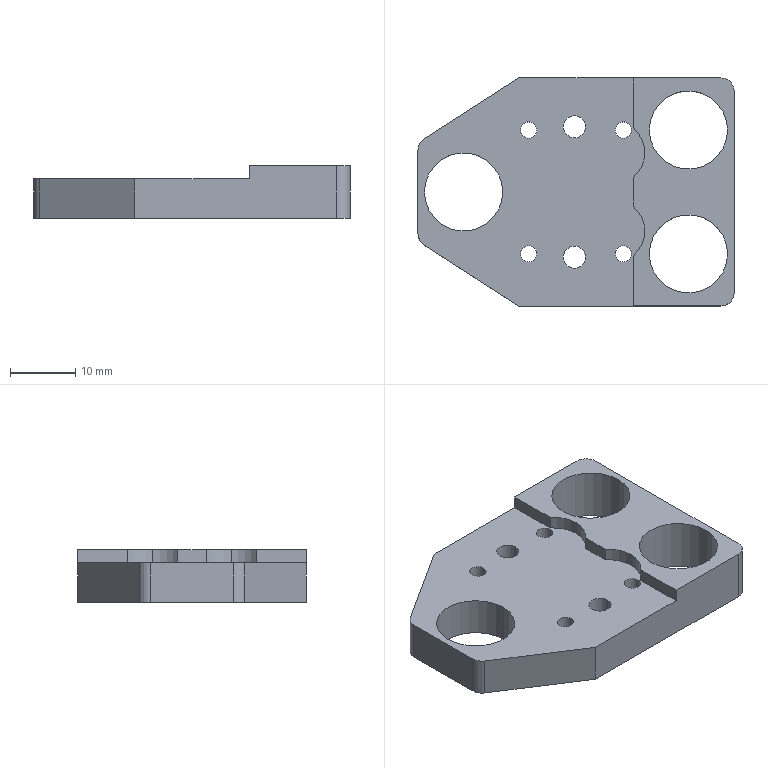Part | STEP file | 11-FG-SB00411 | 1 solid | 44 faces | box 48.5 x 35 x 8 mm | volume 7407 mm3 | cylinder 30 | plane 14 | commonest cylinder face diameters 2.5 x8 12 x6 3.4 x4 4 x4 6.5 x4 10 x4
STEP:
#1=CARTESIAN_POINT('',(-13.75,-9.5,6.));
#2=VERTEX_POINT('',#1);
#3=CARTESIAN_POINT('',(-16.25,-9.5,6.));
#4=VERTEX_POINT('',#3);
#5=CARTESIAN_POINT('',(-15.,-9.5,6.));
#6=DIRECTION('',(0.,0.,-1.));
#7=DIRECTION('',(-1.,0.,0.));
#8=AXIS2_PLACEMENT_3D('',#5,#6,#7);
#9=CIRCLE('',#8,1.25);
#10=EDGE_CURVE('',#2,#4,#9,.T.);
#11=ORIENTED_EDGE('',*,*,#10,.F.);
#12=CARTESIAN_POINT('',(-13.75,-9.5,0.));
#13=VERTEX_POINT('',#12);
#14=CARTESIAN_POINT('',(-13.75,-9.5,0.));
#15=DIRECTION('',(0.,0.,-1.));
#16=VECTOR('',#15,1000.);
#17=LINE('',#14,#16);
#18=EDGE_CURVE('',#2,#13,#17,.T.);
#19=ORIENTED_EDGE('',*,*,#18,.T.);
#20=CARTESIAN_POINT('',(-16.25,-9.5,0.));
#21=VERTEX_POINT('',#20);
#22=CARTESIAN_POINT('',(-15.,-9.5,0.));
#23=DIRECTION('',(0.,0.,-1.));
#24=DIRECTION('',(-1.,0.,0.));
#25=AXIS2_PLACEMENT_3D('',#22,#23,#24);
#26=CIRCLE('',#25,1.25);
#27=EDGE_CURVE('',#13,#21,#26,.T.);
#28=ORIENTED_EDGE('',*,*,#27,.T.);
#29=CARTESIAN_POINT('',(-16.25,-9.5,0.));
#30=DIRECTION('',(0.,0.,-1.));
#31=VECTOR('',#30,1000.);
#32=LINE('',#29,#31);
#33=EDGE_CURVE('',#4,#21,#32,.T.);
#34=ORIENTED_EDGE('',*,*,#33,.F.);
#35=EDGE_LOOP('',(#11,#19,#28,#34));
#36=FACE_OUTER_BOUND('',#35,.T.);
#37=CARTESIAN_POINT('',(-15.,-9.5,0.));
#38=DIRECTION('',(0.,0.,-1.));
#39=DIRECTION('',(-1.,0.,0.));
#40=AXIS2_PLACEMENT_3D('',#37,#38,#39);
#41=CYLINDRICAL_SURFACE('',#40,1.25);
#42=ADVANCED_FACE('',(#36),#41,.F.);
#43=CARTESIAN_POINT('',(-13.75,9.5,6.));
#44=VERTEX_POINT('',#43);
#45=CARTESIAN_POINT('',(-16.25,9.5,6.));
#46=VERTEX_POINT('',#45);
#47=CARTESIAN_POINT('',(-15.,9.5,6.));
#48=DIRECTION('',(0.,0.,-1.));
#49=DIRECTION('',(-1.,0.,0.));
#50=AXIS2_PLACEMENT_3D('',#47,#48,#49);
#51=CIRCLE('',#50,1.25);
#52=EDGE_CURVE('',#44,#46,#51,.T.);
#53=ORIENTED_EDGE('',*,*,#52,.F.);
#54=CARTESIAN_POINT('',(-13.75,9.5,0.));
#55=VERTEX_POINT('',#54);
#56=CARTESIAN_POINT('',(-13.75,9.5,0.));
#57=DIRECTION('',(0.,0.,-1.));
#58=VECTOR('',#57,1000.);
#59=LINE('',#56,#58);
#60=EDGE_CURVE('',#44,#55,#59,.T.);
#61=ORIENTED_EDGE('',*,*,#60,.T.);
#62=CARTESIAN_POINT('',(-16.25,9.5,0.));
#63=VERTEX_POINT('',#62);
#64=CARTESIAN_POINT('',(-15.,9.5,0.));
#65=DIRECTION('',(0.,0.,-1.));
#66=DIRECTION('',(-1.,0.,0.));
#67=AXIS2_PLACEMENT_3D('',#64,#65,#66);
#68=CIRCLE('',#67,1.25);
#69=EDGE_CURVE('',#55,#63,#68,.T.);
#70=ORIENTED_EDGE('',*,*,#69,.T.);
#71=CARTESIAN_POINT('',(-16.25,9.5,0.));
#72=DIRECTION('',(0.,0.,-1.));
#73=VECTOR('',#72,1000.);
#74=LINE('',#71,#73);
#75=EDGE_CURVE('',#46,#63,#74,.T.);
#76=ORIENTED_EDGE('',*,*,#75,.F.);
#77=EDGE_LOOP('',(#53,#61,#70,#76));
#78=FACE_OUTER_BOUND('',#77,.T.);
#79=CARTESIAN_POINT('',(-15.,9.5,0.));
#80=DIRECTION('',(0.,0.,-1.));
#81=DIRECTION('',(-1.,0.,0.));
#82=AXIS2_PLACEMENT_3D('',#79,#80,#81);
#83=CYLINDRICAL_SURFACE('',#82,1.25);
#84=ADVANCED_FACE('',(#78),#83,.F.);
#85=CARTESIAN_POINT('',(-31.,0.,0.));
#86=VERTEX_POINT('',#85);
#87=CARTESIAN_POINT('',(-19.,0.,0.));
#88=VERTEX_POINT('',#87);
#89=CARTESIAN_POINT('',(-25.,0.,0.));
#90=DIRECTION('',(0.,0.,1.));
#91=DIRECTION('',(1.,0.,0.));
#92=AXIS2_PLACEMENT_3D('',#89,#90,#91);
#93=CIRCLE('',#92,6.);
#94=EDGE_CURVE('',#86,#88,#93,.T.);
#95=ORIENTED_EDGE('',*,*,#94,.F.);
#96=CARTESIAN_POINT('',(-31.,0.,6.));
#97=VERTEX_POINT('',#96);
#98=CARTESIAN_POINT('',(-31.,0.,0.));
#99=DIRECTION('',(0.,0.,1.));
#100=VECTOR('',#99,1000.);
#101=LINE('',#98,#100);
#102=EDGE_CURVE('',#86,#97,#101,.T.);
#103=ORIENTED_EDGE('',*,*,#102,.T.);
#104=CARTESIAN_POINT('',(-19.,0.,6.));
#105=VERTEX_POINT('',#104);
#106=CARTESIAN_POINT('',(-25.,0.,6.));
#107=DIRECTION('',(0.,0.,1.));
#108=DIRECTION('',(1.,0.,0.));
#109=AXIS2_PLACEMENT_3D('',#106,#107,#108);
#110=CIRCLE('',#109,6.);
#111=EDGE_CURVE('',#97,#105,#110,.T.);
#112=ORIENTED_EDGE('',*,*,#111,.T.);
#113=CARTESIAN_POINT('',(-19.,0.,0.));
#114=DIRECTION('',(0.,0.,1.));
#115=VECTOR('',#114,1000.);
#116=LINE('',#113,#115);
#117=EDGE_CURVE('',#88,#105,#116,.T.);
#118=ORIENTED_EDGE('',*,*,#117,.F.);
#119=EDGE_LOOP('',(#95,#103,#112,#118));
#120=FACE_OUTER_BOUND('',#119,.T.);
#121=CARTESIAN_POINT('',(-25.,0.,0.));
#122=DIRECTION('',(0.,0.,1.));
#123=DIRECTION('',(1.,0.,0.));
#124=AXIS2_PLACEMENT_3D('',#121,#122,#123);
#125=CYLINDRICAL_SURFACE('',#124,6.);
#126=ADVANCED_FACE('',(#120),#125,.F.);
#127=CARTESIAN_POINT('',(0.75,-9.5,6.));
#128=VERTEX_POINT('',#127);
#129=CARTESIAN_POINT('',(-1.75,-9.5,6.));
#130=VERTEX_POINT('',#129);
#131=CARTESIAN_POINT('',(-0.5,-9.5,6.));
#132=DIRECTION('',(0.,0.,-1.));
#133=DIRECTION('',(-1.,0.,0.));
#134=AXIS2_PLACEMENT_3D('',#131,#132,#133);
#135=CIRCLE('',#134,1.25);
#136=EDGE_CURVE('',#128,#130,#135,.T.);
#137=ORIENTED_EDGE('',*,*,#136,.F.);
#138=CARTESIAN_POINT('',(0.75,-9.5,0.));
#139=VERTEX_POINT('',#138);
#140=CARTESIAN_POINT('',(0.75,-9.5,0.));
#141=DIRECTION('',(0.,0.,-1.));
#142=VECTOR('',#141,1000.);
#143=LINE('',#140,#142);
#144=EDGE_CURVE('',#128,#139,#143,.T.);
#145=ORIENTED_EDGE('',*,*,#144,.T.);
#146=CARTESIAN_POINT('',(-1.75,-9.5,0.));
#147=VERTEX_POINT('',#146);
#148=CARTESIAN_POINT('',(-0.5,-9.5,0.));
#149=DIRECTION('',(0.,0.,-1.));
#150=DIRECTION('',(-1.,0.,0.));
#151=AXIS2_PLACEMENT_3D('',#148,#149,#150);
#152=CIRCLE('',#151,1.25);
#153=EDGE_CURVE('',#139,#147,#152,.T.);
#154=ORIENTED_EDGE('',*,*,#153,.T.);
#155=CARTESIAN_POINT('',(-1.75,-9.5,0.));
#156=DIRECTION('',(0.,0.,-1.));
#157=VECTOR('',#156,1000.);
#158=LINE('',#155,#157);
#159=EDGE_CURVE('',#130,#147,#158,.T.);
#160=ORIENTED_EDGE('',*,*,#159,.F.);
#161=EDGE_LOOP('',(#137,#145,#154,#160));
#162=FACE_OUTER_BOUND('',#161,.T.);
#163=CARTESIAN_POINT('',(-0.5,-9.5,0.));
#164=DIRECTION('',(0.,0.,-1.));
#165=DIRECTION('',(-1.,0.,0.));
#166=AXIS2_PLACEMENT_3D('',#163,#164,#165);
#167=CYLINDRICAL_SURFACE('',#166,1.25);
#168=ADVANCED_FACE('',(#162),#167,.F.);
#169=CARTESIAN_POINT('',(0.75,9.5,6.));
#170=VERTEX_POINT('',#169);
#171=CARTESIAN_POINT('',(-1.75,9.5,6.));
#172=VERTEX_POINT('',#171);
#173=CARTESIAN_POINT('',(-0.5,9.5,6.));
#174=DIRECTION('',(0.,0.,-1.));
#175=DIRECTION('',(-1.,0.,0.));
#176=AXIS2_PLACEMENT_3D('',#173,#174,#175);
#177=CIRCLE('',#176,1.25);
#178=EDGE_CURVE('',#170,#172,#177,.T.);
#179=ORIENTED_EDGE('',*,*,#178,.F.);
#180=CARTESIAN_POINT('',(0.75,9.5,0.));
#181=VERTEX_POINT('',#180);
#182=CARTESIAN_POINT('',(0.75,9.5,0.));
#183=DIRECTION('',(0.,0.,-1.));
#184=VECTOR('',#183,1000.);
#185=LINE('',#182,#184);
#186=EDGE_CURVE('',#170,#181,#185,.T.);
#187=ORIENTED_EDGE('',*,*,#186,.T.);
#188=CARTESIAN_POINT('',(-1.75,9.5,0.));
#189=VERTEX_POINT('',#188);
#190=CARTESIAN_POINT('',(-0.5,9.5,0.));
#191=DIRECTION('',(0.,0.,-1.));
#192=DIRECTION('',(-1.,0.,0.));
#193=AXIS2_PLACEMENT_3D('',#190,#191,#192);
#194=CIRCLE('',#193,1.25);
#195=EDGE_CURVE('',#181,#189,#194,.T.);
#196=ORIENTED_EDGE('',*,*,#195,.T.);
#197=CARTESIAN_POINT('',(-1.75,9.5,0.));
#198=DIRECTION('',(0.,0.,-1.));
#199=VECTOR('',#198,1000.);
#200=LINE('',#197,#199);
#201=EDGE_CURVE('',#172,#189,#200,.T.);
#202=ORIENTED_EDGE('',*,*,#201,.F.);
#203=EDGE_LOOP('',(#179,#187,#196,#202));
#204=FACE_OUTER_BOUND('',#203,.T.);
#205=CARTESIAN_POINT('',(-0.5,9.5,0.));
#206=DIRECTION('',(0.,0.,-1.));
#207=DIRECTION('',(-1.,0.,0.));
#208=AXIS2_PLACEMENT_3D('',#205,#206,#207);
#209=CYLINDRICAL_SURFACE('',#208,1.25);
#210=ADVANCED_FACE('',(#204),#209,.F.);
#211=CARTESIAN_POINT('',(3.5,9.5,0.));
#212=VERTEX_POINT('',#211);
#213=CARTESIAN_POINT('',(15.5,9.5,0.));
#214=VERTEX_POINT('',#213);
#215=CARTESIAN_POINT('',(9.5,9.5,0.));
#216=DIRECTION('',(0.,0.,1.));
#217=DIRECTION('',(-1.,0.,0.));
#218=AXIS2_PLACEMENT_3D('',#215,#216,#217);
#219=CIRCLE('',#218,6.);
#220=EDGE_CURVE('',#212,#214,#219,.T.);
#221=ORIENTED_EDGE('',*,*,#220,.F.);
#222=CARTESIAN_POINT('',(3.5,9.5,8.));
#223=VERTEX_POINT('',#222);
#224=CARTESIAN_POINT('',(3.5,9.5,0.));
#225=DIRECTION('',(0.,0.,1.));
#226=VECTOR('',#225,1000.);
#227=LINE('',#224,#226);
#228=EDGE_CURVE('',#212,#223,#227,.T.);
#229=ORIENTED_EDGE('',*,*,#228,.T.);
#230=CARTESIAN_POINT('',(15.5,9.5,8.));
#231=VERTEX_POINT('',#230);
#232=CARTESIAN_POINT('',(9.5,9.5,8.));
#233=DIRECTION('',(0.,0.,1.));
#234=DIRECTION('',(-1.,0.,0.));
#235=AXIS2_PLACEMENT_3D('',#232,#233,#234);
#236=CIRCLE('',#235,6.);
#237=EDGE_CURVE('',#223,#231,#236,.T.);
#238=ORIENTED_EDGE('',*,*,#237,.T.);
#239=CARTESIAN_POINT('',(15.5,9.5,0.));
#240=DIRECTION('',(0.,0.,1.));
#241=VECTOR('',#240,1000.);
#242=LINE('',#239,#241);
#243=EDGE_CURVE('',#214,#231,#242,.T.);
#244=ORIENTED_EDGE('',*,*,#243,.F.);
#245=EDGE_LOOP('',(#221,#229,#238,#244));
#246=FACE_OUTER_BOUND('',#245,.T.);
#247=CARTESIAN_POINT('',(9.5,9.5,0.));
#248=DIRECTION('',(0.,0.,1.));
#249=DIRECTION('',(1.,0.,0.));
#250=AXIS2_PLACEMENT_3D('',#247,#248,#249);
#251=CYLINDRICAL_SURFACE('',#250,6.);
#252=ADVANCED_FACE('',(#246),#251,.F.);
#253=CARTESIAN_POINT('',(3.5,-9.5,0.));
#254=VERTEX_POINT('',#253);
#255=CARTESIAN_POINT('',(15.5,-9.5,0.));
#256=VERTEX_POINT('',#255);
#257=CARTESIAN_POINT('',(9.5,-9.5,0.));
#258=DIRECTION('',(0.,0.,1.));
#259=DIRECTION('',(1.,0.,0.));
#260=AXIS2_PLACEMENT_3D('',#257,#258,#259);
#261=CIRCLE('',#260,6.);
#262=EDGE_CURVE('',#254,#256,#261,.T.);
#263=ORIENTED_EDGE('',*,*,#262,.F.);
#264=CARTESIAN_POINT('',(3.5,-9.5,8.));
#265=VERTEX_POINT('',#264);
#266=CARTESIAN_POINT('',(3.5,-9.5,0.));
#267=DIRECTION('',(0.,0.,1.));
#268=VECTOR('',#267,1000.);
#269=LINE('',#266,#268);
#270=EDGE_CURVE('',#254,#265,#269,.T.);
#271=ORIENTED_EDGE('',*,*,#270,.T.);
#272=CARTESIAN_POINT('',(15.5,-9.5,8.));
#273=VERTEX_POINT('',#272);
#274=CARTESIAN_POINT('',(9.5,-9.5,8.));
#275=DIRECTION('',(0.,0.,1.));
#276=DIRECTION('',(1.,0.,0.));
#277=AXIS2_PLACEMENT_3D('',#274,#275,#276);
#278=CIRCLE('',#277,6.);
#279=EDGE_CURVE('',#265,#273,#278,.T.);
#280=ORIENTED_EDGE('',*,*,#279,.T.);
#281=CARTESIAN_POINT('',(15.5,-9.5,0.));
#282=DIRECTION('',(0.,0.,1.));
#283=VECTOR('',#282,1000.);
#284=LINE('',#281,#283);
#285=EDGE_CURVE('',#256,#273,#284,.T.);
#286=ORIENTED_EDGE('',*,*,#285,.F.);
#287=EDGE_LOOP('',(#263,#271,#280,#286));
#288=FACE_OUTER_BOUND('',#287,.T.);
#289=CARTESIAN_POINT('',(9.5,-9.5,0.));
#290=DIRECTION('',(0.,0.,1.));
#291=DIRECTION('',(1.,0.,0.));
#292=AXIS2_PLACEMENT_3D('',#289,#290,#291);
#293=CYLINDRICAL_SURFACE('',#292,6.);
#294=ADVANCED_FACE('',(#288),#293,.F.);
#295=CARTESIAN_POINT('',(-4.75,-10.,3.4));
#296=VERTEX_POINT('',#295);
#297=CARTESIAN_POINT('',(-11.25,-10.,3.4));
#298=VERTEX_POINT('',#297);
#299=CARTESIAN_POINT('',(-8.,-10.,3.4));
#300=DIRECTION('',(0.,0.,-1.));
#301=DIRECTION('',(-1.,0.,0.));
#302=AXIS2_PLACEMENT_3D('',#299,#300,#301);
#303=CIRCLE('',#302,3.25);
#304=EDGE_CURVE('',#296,#298,#303,.T.);
#305=ORIENTED_EDGE('',*,*,#304,.F.);
#306=CARTESIAN_POINT('',(-4.75,-10.,0.));
#307=VERTEX_POINT('',#306);
#308=CARTESIAN_POINT('',(-4.75,-10.,0.));
#309=DIRECTION('',(0.,0.,-1.));
#310=VECTOR('',#309,1000.);
#311=LINE('',#308,#310);
#312=EDGE_CURVE('',#296,#307,#311,.T.);
#313=ORIENTED_EDGE('',*,*,#312,.T.);
#314=CARTESIAN_POINT('',(-11.25,-10.,0.));
#315=VERTEX_POINT('',#314);
#316=CARTESIAN_POINT('',(-8.,-10.,0.));
#317=DIRECTION('',(0.,0.,-1.));
#318=DIRECTION('',(-1.,0.,0.));
#319=AXIS2_PLACEMENT_3D('',#316,#317,#318);
#320=CIRCLE('',#319,3.25);
#321=EDGE_CURVE('',#307,#315,#320,.T.);
#322=ORIENTED_EDGE('',*,*,#321,.T.);
#323=CARTESIAN_POINT('',(-11.25,-10.,0.));
#324=DIRECTION('',(0.,0.,-1.));
#325=VECTOR('',#324,1000.);
#326=LINE('',#323,#325);
#327=EDGE_CURVE('',#298,#315,#326,.T.);
#328=ORIENTED_EDGE('',*,*,#327,.F.);
#329=EDGE_LOOP('',(#305,#313,#322,#328));
#330=FACE_OUTER_BOUND('',#329,.T.);
#331=CARTESIAN_POINT('',(-8.,-10.,0.));
#332=DIRECTION('',(0.,0.,-1.));
#333=DIRECTION('',(-1.,0.,0.));
#334=AXIS2_PLACEMENT_3D('',#331,#332,#333);
#335=CYLINDRICAL_SURFACE('',#334,3.25);
#336=ADVANCED_FACE('',(#330),#335,.F.);
#337=CARTESIAN_POINT('',(-6.3,-10.,6.));
#338=VERTEX_POINT('',#337);
#339=CARTESIAN_POINT('',(-9.7,-10.,6.));
#340=VERTEX_POINT('',#339);
#341=CARTESIAN_POINT('',(-8.,-10.,6.));
#342=DIRECTION('',(0.,0.,-1.));
#343=DIRECTION('',(-1.,0.,0.));
#344=AXIS2_PLACEMENT_3D('',#341,#342,#343);
#345=CIRCLE('',#344,1.7);
#346=EDGE_CURVE('',#338,#340,#345,.T.);
#347=ORIENTED_EDGE('',*,*,#346,.F.);
#348=CARTESIAN_POINT('',(-6.3,-10.,3.4));
#349=VERTEX_POINT('',#348);
#350=CARTESIAN_POINT('',(-6.3,-10.,0.));
#351=DIRECTION('',(0.,0.,-1.));
#352=VECTOR('',#351,1000.);
#353=LINE('',#350,#352);
#354=EDGE_CURVE('',#338,#349,#353,.T.);
#355=ORIENTED_EDGE('',*,*,#354,.T.);
#356=CARTESIAN_POINT('',(-9.7,-10.,3.4));
#357=VERTEX_POINT('',#356);
#358=CARTESIAN_POINT('',(-8.,-10.,3.4));
#359=DIRECTION('',(0.,0.,-1.));
#360=DIRECTION('',(-1.,0.,0.));
#361=AXIS2_PLACEMENT_3D('',#358,#359,#360);
#362=CIRCLE('',#361,1.7);
#363=EDGE_CURVE('',#349,#357,#362,.T.);
#364=ORIENTED_EDGE('',*,*,#363,.T.);
#365=CARTESIAN_POINT('',(-9.7,-10.,0.));
#366=DIRECTION('',(0.,0.,-1.));
#367=VECTOR('',#366,1000.);
#368=LINE('',#365,#367);
#369=EDGE_CURVE('',#340,#357,#368,.T.);
#370=ORIENTED_EDGE('',*,*,#369,.F.);
#371=EDGE_LOOP('',(#347,#355,#364,#370));
#372=FACE_OUTER_BOUND('',#371,.T.);
#373=CARTESIAN_POINT('',(-8.,-10.,0.));
#374=DIRECTION('',(0.,0.,-1.));
#375=DIRECTION('',(-1.,0.,0.));
#376=AXIS2_PLACEMENT_3D('',#373,#374,#375);
#377=CYLINDRICAL_SURFACE('',#376,1.7);
#378=ADVANCED_FACE('',(#372),#377,.F.);
#379=CARTESIAN_POINT('',(-4.75,10.,3.4));
#380=VERTEX_POINT('',#379);
#381=CARTESIAN_POINT('',(-11.25,10.,3.4));
#382=VERTEX_POINT('',#381);
#383=CARTESIAN_POINT('',(-8.,10.,3.4));
#384=DIRECTION('',(0.,0.,-1.));
#385=DIRECTION('',(-1.,0.,0.));
#386=AXIS2_PLACEMENT_3D('',#383,#384,#385);
#387=CIRCLE('',#386,3.25);
#388=EDGE_CURVE('',#380,#382,#387,.T.);
#389=ORIENTED_EDGE('',*,*,#388,.F.);
#390=CARTESIAN_POINT('',(-4.75,10.,0.));
#391=VERTEX_POINT('',#390);
#392=CARTESIAN_POINT('',(-4.75,10.,0.));
#393=DIRECTION('',(0.,0.,-1.));
#394=VECTOR('',#393,1000.);
#395=LINE('',#392,#394);
#396=EDGE_CURVE('',#380,#391,#395,.T.);
#397=ORIENTED_EDGE('',*,*,#396,.T.);
#398=CARTESIAN_POINT('',(-11.25,10.,0.));
#399=VERTEX_POINT('',#398);
#400=CARTESIAN_POINT('',(-8.,10.,0.));
#401=DIRECTION('',(0.,0.,-1.));
#402=DIRECTION('',(-1.,0.,0.));
#403=AXIS2_PLACEMENT_3D('',#400,#401,#402);
#404=CIRCLE('',#403,3.25);
#405=EDGE_CURVE('',#391,#399,#404,.T.);
#406=ORIENTED_EDGE('',*,*,#405,.T.);
#407=CARTESIAN_POINT('',(-11.25,10.,0.));
#408=DIRECTION('',(0.,0.,-1.));
#409=VECTOR('',#408,1000.);
#410=LINE('',#407,#409);
#411=EDGE_CURVE('',#382,#399,#410,.T.);
#412=ORIENTED_EDGE('',*,*,#411,.F.);
#413=EDGE_LOOP('',(#389,#397,#406,#412));
#414=FACE_OUTER_BOUND('',#413,.T.);
#415=CARTESIAN_POINT('',(-8.,10.,0.));
#416=DIRECTION('',(0.,0.,-1.));
#417=DIRECTION('',(-1.,0.,0.));
#418=AXIS2_PLACEMENT_3D('',#415,#416,#417);
#419=CYLINDRICAL_SURFACE('',#418,3.25);
#420=ADVANCED_FACE('',(#414),#419,.F.);
#421=CARTESIAN_POINT('',(-6.3,10.,6.));
#422=VERTEX_POINT('',#421);
#423=CARTESIAN_POINT('',(-9.7,10.,6.));
#424=VERTEX_POINT('',#423);
#425=CARTESIAN_POINT('',(-8.,10.,6.));
#426=DIRECTION('',(0.,0.,-1.));
#427=DIRECTION('',(-1.,0.,0.));
#428=AXIS2_PLACEMENT_3D('',#425,#426,#427);
#429=CIRCLE('',#428,1.7);
#430=EDGE_CURVE('',#422,#424,#429,.T.);
#431=ORIENTED_EDGE('',*,*,#430,.F.);
#432=CARTESIAN_POINT('',(-6.3,10.,3.4));
#433=VERTEX_POINT('',#432);
#434=CARTESIAN_POINT('',(-6.3,10.,0.));
#435=DIRECTION('',(0.,0.,-1.));
#436=VECTOR('',#435,1000.);
#437=LINE('',#434,#436);
#438=EDGE_CURVE('',#422,#433,#437,.T.);
#439=ORIENTED_EDGE('',*,*,#438,.T.);
#440=CARTESIAN_POINT('',(-9.7,10.,3.4));
#441=VERTEX_POINT('',#440);
#442=CARTESIAN_POINT('',(-8.,10.,3.4));
#443=DIRECTION('',(0.,0.,-1.));
#444=DIRECTION('',(-1.,0.,0.));
#445=AXIS2_PLACEMENT_3D('',#442,#443,#444);
#446=CIRCLE('',#445,1.7);
#447=EDGE_CURVE('',#433,#441,#446,.T.);
#448=ORIENTED_EDGE('',*,*,#447,.T.);
#449=CARTESIAN_POINT('',(-9.7,10.,0.));
#450=DIRECTION('',(0.,0.,-1.));
#451=VECTOR('',#450,1000.);
#452=LINE('',#449,#451);
#453=EDGE_CURVE('',#424,#441,#452,.T.);
#454=ORIENTED_EDGE('',*,*,#453,.F.);
#455=EDGE_LOOP('',(#431,#439,#448,#454));
#456=FACE_OUTER_BOUND('',#455,.T.);
#457=CARTESIAN_POINT('',(-8.,10.,0.));
#458=DIRECTION('',(0.,0.,-1.));
#459=DIRECTION('',(-1.,0.,0.));
#460=AXIS2_PLACEMENT_3D('',#457,#458,#459);
#461=CYLINDRICAL_SURFACE('',#460,1.7);
#462=ADVANCED_FACE('',(#456),#461,.F.);
#463=CARTESIAN_POINT('',(2.8,-6.,6.));
#464=VERTEX_POINT('',#463);
#465=CARTESIAN_POINT('',(1.,-2.158,6.));
#466=VERTEX_POINT('',#465);
#467=CARTESIAN_POINT('',(-2.2,-6.,6.));
#468=DIRECTION('',(0.,0.,1.));
#469=DIRECTION('',(-1.,0.,0.));
#470=AXIS2_PLACEMENT_3D('',#467,#468,#469);
#471=CIRCLE('',#470,5.);
#472=EDGE_CURVE('',#464,#466,#471,.T.);
#473=ORIENTED_EDGE('',*,*,#472,.F.);
#474=CARTESIAN_POINT('',(2.8,-6.,8.));
#475=VERTEX_POINT('',#474);
#476=CARTESIAN_POINT('',(2.8,-6.,6.));
#477=DIRECTION('',(0.,0.,1.));
#478=VECTOR('',#477,1000.);
#479=LINE('',#476,#478);
#480=EDGE_CURVE('',#464,#475,#479,.T.);
#481=ORIENTED_EDGE('',*,*,#480,.T.);
#482=CARTESIAN_POINT('',(1.,-2.158,8.));
#483=VERTEX_POINT('',#482);
#484=CARTESIAN_POINT('',(-2.2,-6.,8.));
#485=DIRECTION('',(0.,0.,1.));
#486=DIRECTION('',(-1.,0.,0.));
#487=AXIS2_PLACEMENT_3D('',#484,#485,#486);
#488=CIRCLE('',#487,5.);
#489=EDGE_CURVE('',#475,#483,#488,.T.);
#490=ORIENTED_EDGE('',*,*,#489,.T.);
#491=CARTESIAN_POINT('',(1.,-2.158,6.));
#492=DIRECTION('',(0.,0.,1.));
#493=VECTOR('',#492,1000.);
#494=LINE('',#491,#493);
#495=EDGE_CURVE('',#466,#483,#494,.T.);
#496=ORIENTED_EDGE('',*,*,#495,.F.);
#497=EDGE_LOOP('',(#473,#481,#490,#496));
#498=FACE_OUTER_BOUND('',#497,.T.);
#499=CARTESIAN_POINT('',(-2.2,-6.,6.));
#500=DIRECTION('',(0.,0.,1.));
#501=DIRECTION('',(1.,0.,0.));
#502=AXIS2_PLACEMENT_3D('',#499,#500,#501);
#503=CYLINDRICAL_SURFACE('',#502,5.);
#504=ADVANCED_FACE('',(#498),#503,.F.);
#505=CARTESIAN_POINT('',(2.8,6.,6.));
#506=VERTEX_POINT('',#505);
#507=CARTESIAN_POINT('',(1.,9.842,6.));
#508=VERTEX_POINT('',#507);
#509=CARTESIAN_POINT('',(-2.2,6.,6.));
#510=DIRECTION('',(0.,0.,1.));
#511=DIRECTION('',(1.,0.,0.));
#512=AXIS2_PLACEMENT_3D('',#509,#510,#511);
#513=CIRCLE('',#512,5.);
#514=EDGE_CURVE('',#506,#508,#513,.T.);
#515=ORIENTED_EDGE('',*,*,#514,.F.);
#516=CARTESIAN_POINT('',(2.8,6.,8.));
#517=VERTEX_POINT('',#516);
#518=CARTESIAN_POINT('',(2.8,6.,6.));
#519=DIRECTION('',(0.,0.,1.));
#520=VECTOR('',#519,1000.);
#521=LINE('',#518,#520);
#522=EDGE_CURVE('',#506,#517,#521,.T.);
#523=ORIENTED_EDGE('',*,*,#522,.T.);
#524=CARTESIAN_POINT('',(1.,9.842,8.));
#525=VERTEX_POINT('',#524);
#526=CARTESIAN_POINT('',(-2.2,6.,8.));
#527=DIRECTION('',(0.,0.,1.));
#528=DIRECTION('',(1.,0.,0.));
#529=AXIS2_PLACEMENT_3D('',#526,#527,#528);
#530=CIRCLE('',#529,5.);
#531=EDGE_CURVE('',#517,#525,#530,.T.);
#532=ORIENTED_EDGE('',*,*,#531,.T.);
#533=CARTESIAN_POINT('',(1.,9.842,6.));
#534=DIRECTION('',(0.,0.,1.));
#535=VECTOR('',#534,1000.);
#536=LINE('',#533,#535);
#537=EDGE_CURVE('',#508,#525,#536,.T.);
#538=ORIENTED_EDGE('',*,*,#537,.F.);
#539=EDGE_LOOP('',(#515,#523,#532,#538));
#540=FACE_OUTER_BOUND('',#539,.T.);
#541=CARTESIAN_POINT('',(-2.2,6.,6.));
#542=DIRECTION('',(0.,0.,1.));
#543=DIRECTION('',(1.,0.,0.));
#544=AXIS2_PLACEMENT_3D('',#541,#542,#543);
#545=CYLINDRICAL_SURFACE('',#544,5.);
#546=ADVANCED_FACE('',(#540),#545,.F.);
#547=CARTESIAN_POINT('',(1.,2.158,6.));
#548=VERTEX_POINT('',#547);
#549=CARTESIAN_POINT('',(1.,17.5,6.));
#550=DIRECTION('',(0.,-1.,0.));
#551=VECTOR('',#550,1000.);
#552=LINE('',#549,#551);
#553=EDGE_CURVE('',#548,#466,#552,.T.);
#554=ORIENTED_EDGE('',*,*,#553,.T.);
#555=ORIENTED_EDGE('',*,*,#495,.T.);
#556=CARTESIAN_POINT('',(1.,2.158,8.));
#557=VERTEX_POINT('',#556);
#558=CARTESIAN_POINT('',(1.,17.5,8.));
#559=DIRECTION('',(0.,-1.,0.));
#560=VECTOR('',#559,1000.);
#561=LINE('',#558,#560);
#562=EDGE_CURVE('',#557,#483,#561,.T.);
#563=ORIENTED_EDGE('',*,*,#562,.F.);
#564=CARTESIAN_POINT('',(1.,2.158,6.));
#565=DIRECTION('',(0.,0.,-1.));
#566=VECTOR('',#565,1000.);
#567=LINE('',#564,#566);
#568=EDGE_CURVE('',#557,#548,#567,.T.);
#569=ORIENTED_EDGE('',*,*,#568,.T.);
#570=EDGE_LOOP('',(#554,#555,#563,#569));
#571=FACE_OUTER_BOUND('',#570,.T.);
#572=CARTESIAN_POINT('',(1.,17.5,8.));
#573=DIRECTION('',(1.,0.,0.));
#574=DIRECTION('',(0.,0.,-1.));
#575=AXIS2_PLACEMENT_3D('',#572,#573,#574);
#576=PLANE('',#575);
#577=ADVANCED_FACE('',(#571),#576,.F.);
#578=CARTESIAN_POINT('',(1.,17.5,6.));
#579=VERTEX_POINT('',#578);
#580=CARTESIAN_POINT('',(1.,17.5,6.));
#581=DIRECTION('',(0.,-1.,0.));
#582=VECTOR('',#581,1000.);
#583=LINE('',#580,#582);
#584=EDGE_CURVE('',#579,#508,#583,.T.);
#585=ORIENTED_EDGE('',*,*,#584,.T.);
#586=ORIENTED_EDGE('',*,*,#537,.T.);
#587=CARTESIAN_POINT('',(1.,17.5,8.));
#588=VERTEX_POINT('',#587);
#589=CARTESIAN_POINT('',(1.,17.5,8.));
#590=DIRECTION('',(0.,-1.,0.));
#591=VECTOR('',#590,1000.);
#592=LINE('',#589,#591);
#593=EDGE_CURVE('',#588,#525,#592,.T.);
#594=ORIENTED_EDGE('',*,*,#593,.F.);
#595=CARTESIAN_POINT('',(1.,17.5,8.));
#596=DIRECTION('',(0.,0.,1.));
#597=VECTOR('',#596,1000.);
#598=LINE('',#595,#597);
#599=EDGE_CURVE('',#579,#588,#598,.T.);
#600=ORIENTED_EDGE('',*,*,#599,.F.);
#601=EDGE_LOOP('',(#585,#586,#594,#600));
#602=FACE_OUTER_BOUND('',#601,.T.);
#603=CARTESIAN_POINT('',(1.,17.5,8.));
#604=DIRECTION('',(1.,0.,0.));
#605=DIRECTION('',(0.,0.,-1.));
#606=AXIS2_PLACEMENT_3D('',#603,#604,#605);
#607=PLANE('',#606);
#608=ADVANCED_FACE('',(#602),#607,.F.);
#609=CARTESIAN_POINT('',(16.5,-15.5,8.));
#610=VERTEX_POINT('',#609);
#611=CARTESIAN_POINT('',(16.5,15.5,8.));
#612=VERTEX_POINT('',#611);
#613=CARTESIAN_POINT('',(16.5,17.5,8.));
#614=DIRECTION('',(0.,1.,0.));
#615=VECTOR('',#614,1000.);
#616=LINE('',#613,#615);
#617=EDGE_CURVE('',#610,#612,#616,.T.);
#618=ORIENTED_EDGE('',*,*,#617,.F.);
#619=CARTESIAN_POINT('',(16.5,-15.5,0.));
#620=VERTEX_POINT('',#619);
#621=CARTESIAN_POINT('',(16.5,-15.5,8.));
#622=DIRECTION('',(0.,0.,-1.));
#623=VECTOR('',#622,1000.);
#624=LINE('',#621,#623);
#625=EDGE_CURVE('',#610,#620,#624,.T.);
#626=ORIENTED_EDGE('',*,*,#625,.T.);
#627=CARTESIAN_POINT('',(16.5,15.5,0.));
#628=VERTEX_POINT('',#627);
#629=CARTESIAN_POINT('',(16.5,17.5,0.));
#630=DIRECTION('',(0.,1.,0.));
#631=VECTOR('',#630,1000.);
#632=LINE('',#629,#631);
#633=EDGE_CURVE('',#620,#628,#632,.T.);
#634=ORIENTED_EDGE('',*,*,#633,.T.);
#635=CARTESIAN_POINT('',(16.5,15.5,8.));
#636=DIRECTION('',(0.,0.,1.));
#637=VECTOR('',#636,1000.);
#638=LINE('',#635,#637);
#639=EDGE_CURVE('',#628,#612,#638,.T.);
#640=ORIENTED_EDGE('',*,*,#639,.T.);
#641=EDGE_LOOP('',(#618,#626,#634,#640));
#642=FACE_OUTER_BOUND('',#641,.T.);
#643=CARTESIAN_POINT('',(16.5,17.5,8.));
#644=DIRECTION('',(-1.,0.,0.));
#645=DIRECTION('',(0.,-1.,0.));
#646=AXIS2_PLACEMENT_3D('',#643,#644,#645);
#647=PLANE('',#646);
#648=ADVANCED_FACE('',(#642),#647,.F.);
#649=CARTESIAN_POINT('',(14.5,17.5,8.));
#650=VERTEX_POINT('',#649);
#651=CARTESIAN_POINT('',(-16.5,17.5,8.));
#652=DIRECTION('',(-1.,0.,0.));
#653=VECTOR('',#652,1000.);
#654=LINE('',#651,#653);
#655=EDGE_CURVE('',#650,#588,#654,.T.);
#656=ORIENTED_EDGE('',*,*,#655,.F.);
#657=CARTESIAN_POINT('',(14.5,17.5,0.));
#658=VERTEX_POINT('',#657);
#659=CARTESIAN_POINT('',(14.5,17.5,8.));
#660=DIRECTION('',(0.,0.,-1.));
#661=VECTOR('',#660,1000.);
#662=LINE('',#659,#661);
#663=EDGE_CURVE('',#650,#658,#662,.T.);
#664=ORIENTED_EDGE('',*,*,#663,.T.);
#665=CARTESIAN_POINT('',(-16.5,17.5,0.));
#666=VERTEX_POINT('',#665);
#667=CARTESIAN_POINT('',(-16.5,17.5,0.));
#668=DIRECTION('',(-1.,0.,0.));
#669=VECTOR('',#668,1000.);
#670=LINE('',#667,#669);
#671=EDGE_CURVE('',#658,#666,#670,.T.);
#672=ORIENTED_EDGE('',*,*,#671,.T.);
#673=CARTESIAN_POINT('',(-16.5,17.5,6.));
#674=VERTEX_POINT('',#673);
#675=CARTESIAN_POINT('',(-16.5,17.5,0.));
#676=DIRECTION('',(0.,0.,1.));
#677=VECTOR('',#676,1000.);
#678=LINE('',#675,#677);
#679=EDGE_CURVE('',#666,#674,#678,.T.);
#680=ORIENTED_EDGE('',*,*,#679,.T.);
#681=CARTESIAN_POINT('',(-16.5,17.5,6.));
#682=DIRECTION('',(1.,0.,0.));
#683=VECTOR('',#682,1000.);
#684=LINE('',#681,#683);
#685=EDGE_CURVE('',#674,#579,#684,.T.);
#686=ORIENTED_EDGE('',*,*,#685,.T.);
#687=ORIENTED_EDGE('',*,*,#599,.T.);
#688=EDGE_LOOP('',(#656,#664,#672,#680,#686,#687));
#689=FACE_OUTER_BOUND('',#688,.T.);
#690=CARTESIAN_POINT('',(-16.5,17.5,8.));
#691=DIRECTION('',(0.,-1.,0.));
#692=DIRECTION('',(0.,0.,-1.));
#693=AXIS2_PLACEMENT_3D('',#690,#691,#692);
#694=PLANE('',#693);
#695=ADVANCED_FACE('',(#689),#694,.F.);
#696=CARTESIAN_POINT('',(-16.5,-17.5,0.));
#697=VERTEX_POINT('',#696);
#698=CARTESIAN_POINT('',(14.5,-17.5,0.));
#699=VERTEX_POINT('',#698);
#700=CARTESIAN_POINT('',(-16.5,-17.5,0.));
#701=DIRECTION('',(1.,0.,0.));
#702=VECTOR('',#701,1000.);
#703=LINE('',#700,#702);
#704=EDGE_CURVE('',#697,#699,#703,.T.);
#705=ORIENTED_EDGE('',*,*,#704,.T.);
#706=CARTESIAN_POINT('',(14.5,-17.5,8.));
#707=VERTEX_POINT('',#706);
#708=CARTESIAN_POINT('',(14.5,-17.5,8.));
#709=DIRECTION('',(0.,0.,1.));
#710=VECTOR('',#709,1000.);
#711=LINE('',#708,#710);
#712=EDGE_CURVE('',#699,#707,#711,.T.);
#713=ORIENTED_EDGE('',*,*,#712,.T.);
#714=CARTESIAN_POINT('',(1.,-17.5,8.));
#715=VERTEX_POINT('',#714);
#716=CARTESIAN_POINT('',(-16.5,-17.5,8.));
#717=DIRECTION('',(1.,0.,0.));
#718=VECTOR('',#717,1000.);
#719=LINE('',#716,#718);
#720=EDGE_CURVE('',#715,#707,#719,.T.);
#721=ORIENTED_EDGE('',*,*,#720,.F.);
#722=CARTESIAN_POINT('',(1.,-17.5,6.));
#723=VERTEX_POINT('',#722);
#724=CARTESIAN_POINT('',(1.,-17.5,8.));
#725=DIRECTION('',(0.,0.,1.));
#726=VECTOR('',#725,1000.);
#727=LINE('',#724,#726);
#728=EDGE_CURVE('',#723,#715,#727,.T.);
#729=ORIENTED_EDGE('',*,*,#728,.F.);
#730=CARTESIAN_POINT('',(-16.5,-17.5,6.));
#731=VERTEX_POINT('',#730);
#732=CARTESIAN_POINT('',(-16.5,-17.5,6.));
#733=DIRECTION('',(1.,0.,0.));
#734=VECTOR('',#733,1000.);
#735=LINE('',#732,#734);
#736=EDGE_CURVE('',#731,#723,#735,.T.);
#737=ORIENTED_EDGE('',*,*,#736,.F.);
#738=CARTESIAN_POINT('',(-16.5,-17.5,0.));
#739=DIRECTION('',(0.,0.,1.));
#740=VECTOR('',#739,1000.);
#741=LINE('',#738,#740);
#742=EDGE_CURVE('',#697,#731,#741,.T.);
#743=ORIENTED_EDGE('',*,*,#742,.F.);
#744=EDGE_LOOP('',(#705,#713,#721,#729,#737,#743));
#745=FACE_OUTER_BOUND('',#744,.T.);
#746=CARTESIAN_POINT('',(-16.5,-17.5,8.));
#747=DIRECTION('',(0.,1.,0.));
#748=DIRECTION('',(0.,0.,1.));
#749=AXIS2_PLACEMENT_3D('',#746,#747,#748);
#750=PLANE('',#749);
#751=ADVANCED_FACE('',(#745),#750,.F.);
#752=CARTESIAN_POINT('',(9.5,9.5,8.));
#753=DIRECTION('',(0.,0.,1.));
#754=DIRECTION('',(-1.,0.,0.));
#755=AXIS2_PLACEMENT_3D('',#752,#753,#754);
#756=CIRCLE('',#755,6.);
#757=EDGE_CURVE('',#231,#223,#756,.T.);
#758=ORIENTED_EDGE('',*,*,#757,.F.);
#759=ORIENTED_EDGE('',*,*,#237,.F.);
#760=EDGE_LOOP('',(#758,#759));
#761=FACE_BOUND('',#760,.T.);
#762=CARTESIAN_POINT('',(9.5,-9.5,8.));
#763=DIRECTION('',(0.,0.,1.));
#764=DIRECTION('',(1.,0.,0.));
#765=AXIS2_PLACEMENT_3D('',#762,#763,#764);
#766=CIRCLE('',#765,6.);
#767=EDGE_CURVE('',#273,#265,#766,.T.);
#768=ORIENTED_EDGE('',*,*,#767,.F.);
#769=ORIENTED_EDGE('',*,*,#279,.F.);
#770=EDGE_LOOP('',(#768,#769));
#771=FACE_BOUND('',#770,.T.);
#772=ORIENTED_EDGE('',*,*,#720,.T.);
#773=CARTESIAN_POINT('',(14.5,-15.5,8.));
#774=DIRECTION('',(0.,0.,1.));
#775=DIRECTION('',(1.,0.,0.));
#776=AXIS2_PLACEMENT_3D('',#773,#774,#775);
#777=CIRCLE('',#776,2.);
#778=EDGE_CURVE('',#707,#610,#777,.T.);
#779=ORIENTED_EDGE('',*,*,#778,.T.);
#780=ORIENTED_EDGE('',*,*,#617,.T.);
#781=CARTESIAN_POINT('',(14.5,15.5,8.));
#782=DIRECTION('',(0.,0.,1.));
#783=DIRECTION('',(1.,0.,0.));
#784=AXIS2_PLACEMENT_3D('',#781,#782,#783);
#785=CIRCLE('',#784,2.);
#786=EDGE_CURVE('',#612,#650,#785,.T.);
#787=ORIENTED_EDGE('',*,*,#786,.T.);
#788=ORIENTED_EDGE('',*,*,#655,.T.);
#789=ORIENTED_EDGE('',*,*,#593,.T.);
#790=ORIENTED_EDGE('',*,*,#531,.F.);
#791=CARTESIAN_POINT('',(-2.2,6.,8.));
#792=DIRECTION('',(0.,0.,1.));
#793=DIRECTION('',(1.,0.,0.));
#794=AXIS2_PLACEMENT_3D('',#791,#792,#793);
#795=CIRCLE('',#794,5.);
#796=EDGE_CURVE('',#557,#517,#795,.T.);
#797=ORIENTED_EDGE('',*,*,#796,.F.);
#798=ORIENTED_EDGE('',*,*,#562,.T.);
#799=ORIENTED_EDGE('',*,*,#489,.F.);
#800=CARTESIAN_POINT('',(1.,-9.842,8.));
#801=VERTEX_POINT('',#800);
#802=CARTESIAN_POINT('',(-2.2,-6.,8.));
#803=DIRECTION('',(0.,0.,1.));
#804=DIRECTION('',(-1.,0.,0.));
#805=AXIS2_PLACEMENT_3D('',#802,#803,#804);
#806=CIRCLE('',#805,5.);
#807=EDGE_CURVE('',#801,#475,#806,.T.);
#808=ORIENTED_EDGE('',*,*,#807,.F.);
#809=CARTESIAN_POINT('',(1.,17.5,8.));
#810=DIRECTION('',(0.,-1.,0.));
#811=VECTOR('',#810,1000.);
#812=LINE('',#809,#811);
#813=EDGE_CURVE('',#801,#715,#812,.T.);
#814=ORIENTED_EDGE('',*,*,#813,.T.);
#815=EDGE_LOOP('',(#772,#779,#780,#787,#788,#789,#790,#797,#798,#799,#808,#814));
#816=FACE_OUTER_BOUND('',#815,.T.);
#817=CARTESIAN_POINT('',(0.,0.,8.));
#818=DIRECTION('',(0.,0.,1.));
#819=DIRECTION('',(1.,0.,0.));
#820=AXIS2_PLACEMENT_3D('',#817,#818,#819);
#821=PLANE('',#820);
#822=ADVANCED_FACE('',(#761,#771,#816),#821,.T.);
#823=CARTESIAN_POINT('',(-15.,-9.5,0.));
#824=DIRECTION('',(0.,0.,-1.));
#825=DIRECTION('',(-1.,0.,0.));
#826=AXIS2_PLACEMENT_3D('',#823,#824,#825);
#827=CIRCLE('',#826,1.25);
#828=EDGE_CURVE('',#21,#13,#827,.T.);
#829=ORIENTED_EDGE('',*,*,#828,.F.);
#830=ORIENTED_EDGE('',*,*,#27,.F.);
#831=EDGE_LOOP('',(#829,#830));
#832=FACE_BOUND('',#831,.T.);
#833=CARTESIAN_POINT('',(-15.,9.5,0.));
#834=DIRECTION('',(0.,0.,-1.));
#835=DIRECTION('',(-1.,0.,0.));
#836=AXIS2_PLACEMENT_3D('',#833,#834,#835);
#837=CIRCLE('',#836,1.25);
#838=EDGE_CURVE('',#63,#55,#837,.T.);
#839=ORIENTED_EDGE('',*,*,#838,.F.);
#840=ORIENTED_EDGE('',*,*,#69,.F.);
#841=EDGE_LOOP('',(#839,#840));
#842=FACE_BOUND('',#841,.T.);
#843=CARTESIAN_POINT('',(-25.,0.,0.));
#844=DIRECTION('',(0.,0.,1.));
#845=DIRECTION('',(1.,0.,0.));
#846=AXIS2_PLACEMENT_3D('',#843,#844,#845);
#847=CIRCLE('',#846,6.);
#848=EDGE_CURVE('',#88,#86,#847,.T.);
#849=ORIENTED_EDGE('',*,*,#848,.T.);
#850=ORIENTED_EDGE('',*,*,#94,.T.);
#851=EDGE_LOOP('',(#849,#850));
#852=FACE_BOUND('',#851,.T.);
#853=CARTESIAN_POINT('',(-0.5,-9.5,0.));
#854=DIRECTION('',(0.,0.,-1.));
#855=DIRECTION('',(-1.,0.,0.));
#856=AXIS2_PLACEMENT_3D('',#853,#854,#855);
#857=CIRCLE('',#856,1.25);
#858=EDGE_CURVE('',#147,#139,#857,.T.);
#859=ORIENTED_EDGE('',*,*,#858,.F.);
#860=ORIENTED_EDGE('',*,*,#153,.F.);
#861=EDGE_LOOP('',(#859,#860));
#862=FACE_BOUND('',#861,.T.);
#863=CARTESIAN_POINT('',(-0.5,9.5,0.));
#864=DIRECTION('',(0.,0.,-1.));
#865=DIRECTION('',(-1.,0.,0.));
#866=AXIS2_PLACEMENT_3D('',#863,#864,#865);
#867=CIRCLE('',#866,1.25);
#868=EDGE_CURVE('',#189,#181,#867,.T.);
#869=ORIENTED_EDGE('',*,*,#868,.F.);
#870=ORIENTED_EDGE('',*,*,#195,.F.);
#871=EDGE_LOOP('',(#869,#870));
#872=FACE_BOUND('',#871,.T.);
#873=CARTESIAN_POINT('',(9.5,9.5,0.));
#874=DIRECTION('',(0.,0.,1.));
#875=DIRECTION('',(-1.,0.,0.));
#876=AXIS2_PLACEMENT_3D('',#873,#874,#875);
#877=CIRCLE('',#876,6.);
#878=EDGE_CURVE('',#214,#212,#877,.T.);
#879=ORIENTED_EDGE('',*,*,#878,.T.);
#880=ORIENTED_EDGE('',*,*,#220,.T.);
#881=EDGE_LOOP('',(#879,#880));
#882=FACE_BOUND('',#881,.T.);
#883=CARTESIAN_POINT('',(9.5,-9.5,0.));
#884=DIRECTION('',(0.,0.,1.));
#885=DIRECTION('',(1.,0.,0.));
#886=AXIS2_PLACEMENT_3D('',#883,#884,#885);
#887=CIRCLE('',#886,6.);
#888=EDGE_CURVE('',#256,#254,#887,.T.);
#889=ORIENTED_EDGE('',*,*,#888,.T.);
#890=ORIENTED_EDGE('',*,*,#262,.T.);
#891=EDGE_LOOP('',(#889,#890));
#892=FACE_BOUND('',#891,.T.);
#893=CARTESIAN_POINT('',(-8.,-10.,0.));
#894=DIRECTION('',(0.,0.,-1.));
#895=DIRECTION('',(-1.,0.,0.));
#896=AXIS2_PLACEMENT_3D('',#893,#894,#895);
#897=CIRCLE('',#896,3.25);
#898=EDGE_CURVE('',#315,#307,#897,.T.);
#899=ORIENTED_EDGE('',*,*,#898,.F.);
#900=ORIENTED_EDGE('',*,*,#321,.F.);
#901=EDGE_LOOP('',(#899,#900));
#902=FACE_BOUND('',#901,.T.);
#903=CARTESIAN_POINT('',(-8.,10.,0.));
#904=DIRECTION('',(0.,0.,-1.));
#905=DIRECTION('',(-1.,0.,0.));
#906=AXIS2_PLACEMENT_3D('',#903,#904,#905);
#907=CIRCLE('',#906,3.25);
#908=EDGE_CURVE('',#399,#391,#907,.T.);
#909=ORIENTED_EDGE('',*,*,#908,.F.);
#910=ORIENTED_EDGE('',*,*,#405,.F.);
#911=EDGE_LOOP('',(#909,#910));
#912=FACE_BOUND('',#911,.T.);
#913=CARTESIAN_POINT('',(-31.084,-8.091,0.));
#914=VERTEX_POINT('',#913);
#915=CARTESIAN_POINT('',(-32.,-7.5,0.));
#916=DIRECTION('',(-0.8403,0.5421,0.));
#917=VECTOR('',#916,1000.);
#918=LINE('',#915,#917);
#919=EDGE_CURVE('',#697,#914,#918,.T.);
#920=ORIENTED_EDGE('',*,*,#919,.T.);
#921=CARTESIAN_POINT('',(-32.,-6.41,0.));
#922=VERTEX_POINT('',#921);
#923=CARTESIAN_POINT('',(-30.,-6.41,0.));
#924=DIRECTION('',(0.,0.,-1.));
#925=DIRECTION('',(1.,0.,0.));
#926=AXIS2_PLACEMENT_3D('',#923,#924,#925);
#927=CIRCLE('',#926,2.);
#928=EDGE_CURVE('',#914,#922,#927,.T.);
#929=ORIENTED_EDGE('',*,*,#928,.T.);
#930=CARTESIAN_POINT('',(-32.,6.41,0.));
#931=VERTEX_POINT('',#930);
#932=CARTESIAN_POINT('',(-32.,17.5,0.));
#933=DIRECTION('',(0.,-1.,0.));
#934=VECTOR('',#933,1000.);
#935=LINE('',#932,#934);
#936=EDGE_CURVE('',#931,#922,#935,.T.);
#937=ORIENTED_EDGE('',*,*,#936,.F.);
#938=CARTESIAN_POINT('',(-31.084,8.091,0.));
#939=VERTEX_POINT('',#938);
#940=CARTESIAN_POINT('',(-30.,6.41,0.));
#941=DIRECTION('',(0.,0.,-1.));
#942=DIRECTION('',(1.,0.,0.));
#943=AXIS2_PLACEMENT_3D('',#940,#941,#942);
#944=CIRCLE('',#943,2.);
#945=EDGE_CURVE('',#931,#939,#944,.T.);
#946=ORIENTED_EDGE('',*,*,#945,.T.);
#947=CARTESIAN_POINT('',(-32.,7.5,0.));
#948=DIRECTION('',(0.8403,0.5421,0.));
#949=VECTOR('',#948,1000.);
#950=LINE('',#947,#949);
#951=EDGE_CURVE('',#939,#666,#950,.T.);
#952=ORIENTED_EDGE('',*,*,#951,.T.);
#953=ORIENTED_EDGE('',*,*,#671,.F.);
#954=CARTESIAN_POINT('',(14.5,15.5,0.));
#955=DIRECTION('',(0.,0.,-1.));
#956=DIRECTION('',(1.,0.,0.));
#957=AXIS2_PLACEMENT_3D('',#954,#955,#956);
#958=CIRCLE('',#957,2.);
#959=EDGE_CURVE('',#658,#628,#958,.T.);
#960=ORIENTED_EDGE('',*,*,#959,.T.);
#961=ORIENTED_EDGE('',*,*,#633,.F.);
#962=CARTESIAN_POINT('',(14.5,-15.5,0.));
#963=DIRECTION('',(0.,0.,-1.));
#964=DIRECTION('',(1.,0.,0.));
#965=AXIS2_PLACEMENT_3D('',#962,#963,#964);
#966=CIRCLE('',#965,2.);
#967=EDGE_CURVE('',#620,#699,#966,.T.);
#968=ORIENTED_EDGE('',*,*,#967,.T.);
#969=ORIENTED_EDGE('',*,*,#704,.F.);
#970=EDGE_LOOP('',(#920,#929,#937,#946,#952,#953,#960,#961,#968,#969));
#971=FACE_OUTER_BOUND('',#970,.T.);
#972=CARTESIAN_POINT('',(0.,0.,0.));
#973=DIRECTION('',(0.,0.,1.));
#974=DIRECTION('',(1.,0.,0.));
#975=AXIS2_PLACEMENT_3D('',#972,#973,#974);
#976=PLANE('',#975);
#977=ADVANCED_FACE('',(#832,#842,#852,#862,#872,#882,#892,#902,#912,#971),#976,.F.);
#978=ORIENTED_EDGE('',*,*,#813,.F.);
#979=CARTESIAN_POINT('',(1.,-9.842,6.));
#980=VERTEX_POINT('',#979);
#981=CARTESIAN_POINT('',(1.,-9.842,6.));
#982=DIRECTION('',(0.,0.,-1.));
#983=VECTOR('',#982,1000.);
#984=LINE('',#981,#983);
#985=EDGE_CURVE('',#801,#980,#984,.T.);
#986=ORIENTED_EDGE('',*,*,#985,.T.);
#987=CARTESIAN_POINT('',(1.,17.5,6.));
#988=DIRECTION('',(0.,-1.,0.));
#989=VECTOR('',#988,1000.);
#990=LINE('',#987,#989);
#991=EDGE_CURVE('',#980,#723,#990,.T.);
#992=ORIENTED_EDGE('',*,*,#991,.T.);
#993=ORIENTED_EDGE('',*,*,#728,.T.);
#994=EDGE_LOOP('',(#978,#986,#992,#993));
#995=FACE_OUTER_BOUND('',#994,.T.);
#996=CARTESIAN_POINT('',(1.,17.5,8.));
#997=DIRECTION('',(1.,0.,0.));
#998=DIRECTION('',(0.,0.,-1.));
#999=AXIS2_PLACEMENT_3D('',#996,#997,#998);
#1000=PLANE('',#999);
#1001=ADVANCED_FACE('',(#995),#1000,.F.);
#1002=CARTESIAN_POINT('',(-15.,-9.5,6.));
#1003=DIRECTION('',(0.,0.,-1.));
#1004=DIRECTION('',(-1.,0.,0.));
#1005=AXIS2_PLACEMENT_3D('',#1002,#1003,#1004);
#1006=CIRCLE('',#1005,1.25);
#1007=EDGE_CURVE('',#4,#2,#1006,.T.);
#1008=ORIENTED_EDGE('',*,*,#1007,.T.);
#1009=ORIENTED_EDGE('',*,*,#10,.T.);
#1010=EDGE_LOOP('',(#1008,#1009));
#1011=FACE_BOUND('',#1010,.T.);
#1012=CARTESIAN_POINT('',(-15.,9.5,6.));
#1013=DIRECTION('',(0.,0.,-1.));
#1014=DIRECTION('',(-1.,0.,0.));
#1015=AXIS2_PLACEMENT_3D('',#1012,#1013,#1014);
#1016=CIRCLE('',#1015,1.25);
#1017=EDGE_CURVE('',#46,#44,#1016,.T.);
#1018=ORIENTED_EDGE('',*,*,#1017,.T.);
#1019=ORIENTED_EDGE('',*,*,#52,.T.);
#1020=EDGE_LOOP('',(#1018,#1019));
#1021=FACE_BOUND('',#1020,.T.);
#1022=CARTESIAN_POINT('',(-25.,0.,6.));
#1023=DIRECTION('',(0.,0.,1.));
#1024=DIRECTION('',(1.,0.,0.));
#1025=AXIS2_PLACEMENT_3D('',#1022,#1023,#1024);
#1026=CIRCLE('',#1025,6.);
#1027=EDGE_CURVE('',#105,#97,#1026,.T.);
#1028=ORIENTED_EDGE('',*,*,#1027,.F.);
#1029=ORIENTED_EDGE('',*,*,#111,.F.);
#1030=EDGE_LOOP('',(#1028,#1029));
#1031=FACE_BOUND('',#1030,.T.);
#1032=CARTESIAN_POINT('',(-0.5,-9.5,6.));
#1033=DIRECTION('',(0.,0.,-1.));
#1034=DIRECTION('',(-1.,0.,0.));
#1035=AXIS2_PLACEMENT_3D('',#1032,#1033,#1034);
#1036=CIRCLE('',#1035,1.25);
#1037=EDGE_CURVE('',#130,#128,#1036,.T.);
#1038=ORIENTED_EDGE('',*,*,#1037,.T.);
#1039=ORIENTED_EDGE('',*,*,#136,.T.);
#1040=EDGE_LOOP('',(#1038,#1039));
#1041=FACE_BOUND('',#1040,.T.);
#1042=CARTESIAN_POINT('',(-0.5,9.5,6.));
#1043=DIRECTION('',(0.,0.,-1.));
#1044=DIRECTION('',(-1.,0.,0.));
#1045=AXIS2_PLACEMENT_3D('',#1042,#1043,#1044);
#1046=CIRCLE('',#1045,1.25);
#1047=EDGE_CURVE('',#172,#170,#1046,.T.);
#1048=ORIENTED_EDGE('',*,*,#1047,.T.);
#1049=ORIENTED_EDGE('',*,*,#178,.T.);
#1050=EDGE_LOOP('',(#1048,#1049));
#1051=FACE_BOUND('',#1050,.T.);
#1052=CARTESIAN_POINT('',(-8.,-10.,6.));
#1053=DIRECTION('',(0.,0.,-1.));
#1054=DIRECTION('',(-1.,0.,0.));
#1055=AXIS2_PLACEMENT_3D('',#1052,#1053,#1054);
#1056=CIRCLE('',#1055,1.7);
#1057=EDGE_CURVE('',#340,#338,#1056,.T.);
#1058=ORIENTED_EDGE('',*,*,#1057,.T.);
#1059=ORIENTED_EDGE('',*,*,#346,.T.);
#1060=EDGE_LOOP('',(#1058,#1059));
#1061=FACE_BOUND('',#1060,.T.);
#1062=CARTESIAN_POINT('',(-8.,10.,6.));
#1063=DIRECTION('',(0.,0.,-1.));
#1064=DIRECTION('',(-1.,0.,0.));
#1065=AXIS2_PLACEMENT_3D('',#1062,#1063,#1064);
#1066=CIRCLE('',#1065,1.7);
#1067=EDGE_CURVE('',#424,#422,#1066,.T.);
#1068=ORIENTED_EDGE('',*,*,#1067,.T.);
#1069=ORIENTED_EDGE('',*,*,#430,.T.);
#1070=EDGE_LOOP('',(#1068,#1069));
#1071=FACE_BOUND('',#1070,.T.);
#1072=CARTESIAN_POINT('',(-32.,-6.41,6.));
#1073=VERTEX_POINT('',#1072);
#1074=CARTESIAN_POINT('',(-32.,6.41,6.));
#1075=VERTEX_POINT('',#1074);
#1076=CARTESIAN_POINT('',(-32.,17.5,6.));
#1077=DIRECTION('',(0.,1.,0.));
#1078=VECTOR('',#1077,1000.);
#1079=LINE('',#1076,#1078);
#1080=EDGE_CURVE('',#1073,#1075,#1079,.T.);
#1081=ORIENTED_EDGE('',*,*,#1080,.F.);
#1082=CARTESIAN_POINT('',(-31.084,-8.091,6.));
#1083=VERTEX_POINT('',#1082);
#1084=CARTESIAN_POINT('',(-30.,-6.41,6.));
#1085=DIRECTION('',(0.,0.,1.));
#1086=DIRECTION('',(-1.,0.,0.));
#1087=AXIS2_PLACEMENT_3D('',#1084,#1085,#1086);
#1088=CIRCLE('',#1087,2.);
#1089=EDGE_CURVE('',#1073,#1083,#1088,.T.);
#1090=ORIENTED_EDGE('',*,*,#1089,.T.);
#1091=CARTESIAN_POINT('',(-32.,-7.5,6.));
#1092=DIRECTION('',(-0.8403,0.5421,0.));
#1093=VECTOR('',#1092,1000.);
#1094=LINE('',#1091,#1093);
#1095=EDGE_CURVE('',#731,#1083,#1094,.T.);
#1096=ORIENTED_EDGE('',*,*,#1095,.F.);
#1097=ORIENTED_EDGE('',*,*,#736,.T.);
#1098=ORIENTED_EDGE('',*,*,#991,.F.);
#1099=CARTESIAN_POINT('',(-2.2,-6.,6.));
#1100=DIRECTION('',(0.,0.,1.));
#1101=DIRECTION('',(-1.,0.,0.));
#1102=AXIS2_PLACEMENT_3D('',#1099,#1100,#1101);
#1103=CIRCLE('',#1102,5.);
#1104=EDGE_CURVE('',#980,#464,#1103,.T.);
#1105=ORIENTED_EDGE('',*,*,#1104,.T.);
#1106=ORIENTED_EDGE('',*,*,#472,.T.);
#1107=ORIENTED_EDGE('',*,*,#553,.F.);
#1108=CARTESIAN_POINT('',(-2.2,6.,6.));
#1109=DIRECTION('',(0.,0.,1.));
#1110=DIRECTION('',(1.,0.,0.));
#1111=AXIS2_PLACEMENT_3D('',#1108,#1109,#1110);
#1112=CIRCLE('',#1111,5.);
#1113=EDGE_CURVE('',#548,#506,#1112,.T.);
#1114=ORIENTED_EDGE('',*,*,#1113,.T.);
#1115=ORIENTED_EDGE('',*,*,#514,.T.);
#1116=ORIENTED_EDGE('',*,*,#584,.F.);
#1117=ORIENTED_EDGE('',*,*,#685,.F.);
#1118=CARTESIAN_POINT('',(-31.084,8.091,6.));
#1119=VERTEX_POINT('',#1118);
#1120=CARTESIAN_POINT('',(-32.,7.5,6.));
#1121=DIRECTION('',(0.8403,0.5421,0.));
#1122=VECTOR('',#1121,1000.);
#1123=LINE('',#1120,#1122);
#1124=EDGE_CURVE('',#1119,#674,#1123,.T.);
#1125=ORIENTED_EDGE('',*,*,#1124,.F.);
#1126=CARTESIAN_POINT('',(-30.,6.41,6.));
#1127=DIRECTION('',(0.,0.,1.));
#1128=DIRECTION('',(-1.,0.,0.));
#1129=AXIS2_PLACEMENT_3D('',#1126,#1127,#1128);
#1130=CIRCLE('',#1129,2.);
#1131=EDGE_CURVE('',#1119,#1075,#1130,.T.);
#1132=ORIENTED_EDGE('',*,*,#1131,.T.);
#1133=EDGE_LOOP('',(#1081,#1090,#1096,#1097,#1098,#1105,#1106,#1107,#1114,#1115,#1116,#1117,#1125,#1132));
#1134=FACE_OUTER_BOUND('',#1133,.T.);
#1135=CARTESIAN_POINT('',(-16.5,17.5,6.));
#1136=DIRECTION('',(0.,0.,-1.));
#1137=DIRECTION('',(-1.,0.,0.));
#1138=AXIS2_PLACEMENT_3D('',#1135,#1136,#1137);
#1139=PLANE('',#1138);
#1140=ADVANCED_FACE('',(#1011,#1021,#1031,#1041,#1051,#1061,#1071,#1134),#1139,.F.);
#1141=ORIENTED_EDGE('',*,*,#522,.F.);
#1142=ORIENTED_EDGE('',*,*,#1113,.F.);
#1143=ORIENTED_EDGE('',*,*,#568,.F.);
#1144=ORIENTED_EDGE('',*,*,#796,.T.);
#1145=EDGE_LOOP('',(#1141,#1142,#1143,#1144));
#1146=FACE_OUTER_BOUND('',#1145,.T.);
#1147=CARTESIAN_POINT('',(-2.2,6.,6.));
#1148=DIRECTION('',(0.,0.,1.));
#1149=DIRECTION('',(1.,0.,0.));
#1150=AXIS2_PLACEMENT_3D('',#1147,#1148,#1149);
#1151=CYLINDRICAL_SURFACE('',#1150,5.);
#1152=ADVANCED_FACE('',(#1146),#1151,.F.);
#1153=ORIENTED_EDGE('',*,*,#480,.F.);
#1154=ORIENTED_EDGE('',*,*,#1104,.F.);
#1155=ORIENTED_EDGE('',*,*,#985,.F.);
#1156=ORIENTED_EDGE('',*,*,#807,.T.);
#1157=EDGE_LOOP('',(#1153,#1154,#1155,#1156));
#1158=FACE_OUTER_BOUND('',#1157,.T.);
#1159=CARTESIAN_POINT('',(-2.2,-6.,6.));
#1160=DIRECTION('',(0.,0.,1.));
#1161=DIRECTION('',(1.,0.,0.));
#1162=AXIS2_PLACEMENT_3D('',#1159,#1160,#1161);
#1163=CYLINDRICAL_SURFACE('',#1162,5.);
#1164=ADVANCED_FACE('',(#1158),#1163,.F.);
#1165=ORIENTED_EDGE('',*,*,#438,.F.);
#1166=ORIENTED_EDGE('',*,*,#1067,.F.);
#1167=ORIENTED_EDGE('',*,*,#453,.T.);
#1168=CARTESIAN_POINT('',(-8.,10.,3.4));
#1169=DIRECTION('',(0.,0.,-1.));
#1170=DIRECTION('',(-1.,0.,0.));
#1171=AXIS2_PLACEMENT_3D('',#1168,#1169,#1170);
#1172=CIRCLE('',#1171,1.7);
#1173=EDGE_CURVE('',#441,#433,#1172,.T.);
#1174=ORIENTED_EDGE('',*,*,#1173,.T.);
#1175=EDGE_LOOP('',(#1165,#1166,#1167,#1174));
#1176=FACE_OUTER_BOUND('',#1175,.T.);
#1177=CARTESIAN_POINT('',(-8.,10.,0.));
#1178=DIRECTION('',(0.,0.,-1.));
#1179=DIRECTION('',(-1.,0.,0.));
#1180=AXIS2_PLACEMENT_3D('',#1177,#1178,#1179);
#1181=CYLINDRICAL_SURFACE('',#1180,1.7);
#1182=ADVANCED_FACE('',(#1176),#1181,.F.);
#1183=ORIENTED_EDGE('',*,*,#1173,.F.);
#1184=ORIENTED_EDGE('',*,*,#447,.F.);
#1185=EDGE_LOOP('',(#1183,#1184));
#1186=FACE_BOUND('',#1185,.T.);
#1187=CARTESIAN_POINT('',(-8.,10.,3.4));
#1188=DIRECTION('',(0.,0.,-1.));
#1189=DIRECTION('',(-1.,0.,0.));
#1190=AXIS2_PLACEMENT_3D('',#1187,#1188,#1189);
#1191=CIRCLE('',#1190,3.25);
#1192=EDGE_CURVE('',#382,#380,#1191,.T.);
#1193=ORIENTED_EDGE('',*,*,#1192,.T.);
#1194=ORIENTED_EDGE('',*,*,#388,.T.);
#1195=EDGE_LOOP('',(#1193,#1194));
#1196=FACE_OUTER_BOUND('',#1195,.T.);
#1197=CARTESIAN_POINT('',(-6.3,10.,3.4));
#1198=DIRECTION('',(0.,0.,1.));
#1199=DIRECTION('',(1.,0.,0.));
#1200=AXIS2_PLACEMENT_3D('',#1197,#1198,#1199);
#1201=PLANE('',#1200);
#1202=ADVANCED_FACE('',(#1186,#1196),#1201,.F.);
#1203=ORIENTED_EDGE('',*,*,#396,.F.);
#1204=ORIENTED_EDGE('',*,*,#1192,.F.);
#1205=ORIENTED_EDGE('',*,*,#411,.T.);
#1206=ORIENTED_EDGE('',*,*,#908,.T.);
#1207=EDGE_LOOP('',(#1203,#1204,#1205,#1206));
#1208=FACE_OUTER_BOUND('',#1207,.T.);
#1209=CARTESIAN_POINT('',(-8.,10.,0.));
#1210=DIRECTION('',(0.,0.,-1.));
#1211=DIRECTION('',(-1.,0.,0.));
#1212=AXIS2_PLACEMENT_3D('',#1209,#1210,#1211);
#1213=CYLINDRICAL_SURFACE('',#1212,3.25);
#1214=ADVANCED_FACE('',(#1208),#1213,.F.);
#1215=ORIENTED_EDGE('',*,*,#354,.F.);
#1216=ORIENTED_EDGE('',*,*,#1057,.F.);
#1217=ORIENTED_EDGE('',*,*,#369,.T.);
#1218=CARTESIAN_POINT('',(-8.,-10.,3.4));
#1219=DIRECTION('',(0.,0.,-1.));
#1220=DIRECTION('',(-1.,0.,0.));
#1221=AXIS2_PLACEMENT_3D('',#1218,#1219,#1220);
#1222=CIRCLE('',#1221,1.7);
#1223=EDGE_CURVE('',#357,#349,#1222,.T.);
#1224=ORIENTED_EDGE('',*,*,#1223,.T.);
#1225=EDGE_LOOP('',(#1215,#1216,#1217,#1224));
#1226=FACE_OUTER_BOUND('',#1225,.T.);
#1227=CARTESIAN_POINT('',(-8.,-10.,0.));
#1228=DIRECTION('',(0.,0.,-1.));
#1229=DIRECTION('',(-1.,0.,0.));
#1230=AXIS2_PLACEMENT_3D('',#1227,#1228,#1229);
#1231=CYLINDRICAL_SURFACE('',#1230,1.7);
#1232=ADVANCED_FACE('',(#1226),#1231,.F.);
#1233=ORIENTED_EDGE('',*,*,#1223,.F.);
#1234=ORIENTED_EDGE('',*,*,#363,.F.);
#1235=EDGE_LOOP('',(#1233,#1234));
#1236=FACE_BOUND('',#1235,.T.);
#1237=CARTESIAN_POINT('',(-8.,-10.,3.4));
#1238=DIRECTION('',(0.,0.,-1.));
#1239=DIRECTION('',(-1.,0.,0.));
#1240=AXIS2_PLACEMENT_3D('',#1237,#1238,#1239);
#1241=CIRCLE('',#1240,3.25);
#1242=EDGE_CURVE('',#298,#296,#1241,.T.);
#1243=ORIENTED_EDGE('',*,*,#1242,.T.);
#1244=ORIENTED_EDGE('',*,*,#304,.T.);
#1245=EDGE_LOOP('',(#1243,#1244));
#1246=FACE_OUTER_BOUND('',#1245,.T.);
#1247=CARTESIAN_POINT('',(-6.3,-10.,3.4));
#1248=DIRECTION('',(0.,0.,1.));
#1249=DIRECTION('',(1.,0.,0.));
#1250=AXIS2_PLACEMENT_3D('',#1247,#1248,#1249);
#1251=PLANE('',#1250);
#1252=ADVANCED_FACE('',(#1236,#1246),#1251,.F.);
#1253=ORIENTED_EDGE('',*,*,#312,.F.);
#1254=ORIENTED_EDGE('',*,*,#1242,.F.);
#1255=ORIENTED_EDGE('',*,*,#327,.T.);
#1256=ORIENTED_EDGE('',*,*,#898,.T.);
#1257=EDGE_LOOP('',(#1253,#1254,#1255,#1256));
#1258=FACE_OUTER_BOUND('',#1257,.T.);
#1259=CARTESIAN_POINT('',(-8.,-10.,0.));
#1260=DIRECTION('',(0.,0.,-1.));
#1261=DIRECTION('',(-1.,0.,0.));
#1262=AXIS2_PLACEMENT_3D('',#1259,#1260,#1261);
#1263=CYLINDRICAL_SURFACE('',#1262,3.25);
#1264=ADVANCED_FACE('',(#1258),#1263,.F.);
#1265=ORIENTED_EDGE('',*,*,#270,.F.);
#1266=ORIENTED_EDGE('',*,*,#888,.F.);
#1267=ORIENTED_EDGE('',*,*,#285,.T.);
#1268=ORIENTED_EDGE('',*,*,#767,.T.);
#1269=EDGE_LOOP('',(#1265,#1266,#1267,#1268));
#1270=FACE_OUTER_BOUND('',#1269,.T.);
#1271=CARTESIAN_POINT('',(9.5,-9.5,0.));
#1272=DIRECTION('',(0.,0.,1.));
#1273=DIRECTION('',(1.,0.,0.));
#1274=AXIS2_PLACEMENT_3D('',#1271,#1272,#1273);
#1275=CYLINDRICAL_SURFACE('',#1274,6.);
#1276=ADVANCED_FACE('',(#1270),#1275,.F.);
#1277=ORIENTED_EDGE('',*,*,#228,.F.);
#1278=ORIENTED_EDGE('',*,*,#878,.F.);
#1279=ORIENTED_EDGE('',*,*,#243,.T.);
#1280=ORIENTED_EDGE('',*,*,#757,.T.);
#1281=EDGE_LOOP('',(#1277,#1278,#1279,#1280));
#1282=FACE_OUTER_BOUND('',#1281,.T.);
#1283=CARTESIAN_POINT('',(9.5,9.5,0.));
#1284=DIRECTION('',(0.,0.,1.));
#1285=DIRECTION('',(1.,0.,0.));
#1286=AXIS2_PLACEMENT_3D('',#1283,#1284,#1285);
#1287=CYLINDRICAL_SURFACE('',#1286,6.);
#1288=ADVANCED_FACE('',(#1282),#1287,.F.);
#1289=ORIENTED_EDGE('',*,*,#186,.F.);
#1290=ORIENTED_EDGE('',*,*,#1047,.F.);
#1291=ORIENTED_EDGE('',*,*,#201,.T.);
#1292=ORIENTED_EDGE('',*,*,#868,.T.);
#1293=EDGE_LOOP('',(#1289,#1290,#1291,#1292));
#1294=FACE_OUTER_BOUND('',#1293,.T.);
#1295=CARTESIAN_POINT('',(-0.5,9.5,0.));
#1296=DIRECTION('',(0.,0.,-1.));
#1297=DIRECTION('',(-1.,0.,0.));
#1298=AXIS2_PLACEMENT_3D('',#1295,#1296,#1297);
#1299=CYLINDRICAL_SURFACE('',#1298,1.25);
#1300=ADVANCED_FACE('',(#1294),#1299,.F.);
#1301=ORIENTED_EDGE('',*,*,#144,.F.);
#1302=ORIENTED_EDGE('',*,*,#1037,.F.);
#1303=ORIENTED_EDGE('',*,*,#159,.T.);
#1304=ORIENTED_EDGE('',*,*,#858,.T.);
#1305=EDGE_LOOP('',(#1301,#1302,#1303,#1304));
#1306=FACE_OUTER_BOUND('',#1305,.T.);
#1307=CARTESIAN_POINT('',(-0.5,-9.5,0.));
#1308=DIRECTION('',(0.,0.,-1.));
#1309=DIRECTION('',(-1.,0.,0.));
#1310=AXIS2_PLACEMENT_3D('',#1307,#1308,#1309);
#1311=CYLINDRICAL_SURFACE('',#1310,1.25);
#1312=ADVANCED_FACE('',(#1306),#1311,.F.);
#1313=ORIENTED_EDGE('',*,*,#936,.T.);
#1314=CARTESIAN_POINT('',(-32.,-6.41,0.));
#1315=DIRECTION('',(0.,0.,1.));
#1316=VECTOR('',#1315,1000.);
#1317=LINE('',#1314,#1316);
#1318=EDGE_CURVE('',#922,#1073,#1317,.T.);
#1319=ORIENTED_EDGE('',*,*,#1318,.T.);
#1320=ORIENTED_EDGE('',*,*,#1080,.T.);
#1321=CARTESIAN_POINT('',(-32.,6.41,0.));
#1322=DIRECTION('',(0.,0.,-1.));
#1323=VECTOR('',#1322,1000.);
#1324=LINE('',#1321,#1323);
#1325=EDGE_CURVE('',#1075,#931,#1324,.T.);
#1326=ORIENTED_EDGE('',*,*,#1325,.T.);
#1327=EDGE_LOOP('',(#1313,#1319,#1320,#1326));
#1328=FACE_OUTER_BOUND('',#1327,.T.);
#1329=CARTESIAN_POINT('',(-32.,0.,0.));
#1330=DIRECTION('',(1.,0.,0.));
#1331=DIRECTION('',(0.,1.,0.));
#1332=AXIS2_PLACEMENT_3D('',#1329,#1330,#1331);
#1333=PLANE('',#1332);
#1334=ADVANCED_FACE('',(#1328),#1333,.F.);
#1335=ORIENTED_EDGE('',*,*,#102,.F.);
#1336=ORIENTED_EDGE('',*,*,#848,.F.);
#1337=ORIENTED_EDGE('',*,*,#117,.T.);
#1338=ORIENTED_EDGE('',*,*,#1027,.T.);
#1339=EDGE_LOOP('',(#1335,#1336,#1337,#1338));
#1340=FACE_OUTER_BOUND('',#1339,.T.);
#1341=CARTESIAN_POINT('',(-25.,0.,0.));
#1342=DIRECTION('',(0.,0.,1.));
#1343=DIRECTION('',(1.,0.,0.));
#1344=AXIS2_PLACEMENT_3D('',#1341,#1342,#1343);
#1345=CYLINDRICAL_SURFACE('',#1344,6.);
#1346=ADVANCED_FACE('',(#1340),#1345,.F.);
#1347=ORIENTED_EDGE('',*,*,#951,.F.);
#1348=CARTESIAN_POINT('',(-31.084,8.091,0.));
#1349=DIRECTION('',(0.,0.,1.));
#1350=VECTOR('',#1349,1000.);
#1351=LINE('',#1348,#1350);
#1352=EDGE_CURVE('',#939,#1119,#1351,.T.);
#1353=ORIENTED_EDGE('',*,*,#1352,.T.);
#1354=ORIENTED_EDGE('',*,*,#1124,.T.);
#1355=ORIENTED_EDGE('',*,*,#679,.F.);
#1356=EDGE_LOOP('',(#1347,#1353,#1354,#1355));
#1357=FACE_OUTER_BOUND('',#1356,.T.);
#1358=CARTESIAN_POINT('',(-32.,7.5,0.));
#1359=DIRECTION('',(0.5421,-0.8403,0.));
#1360=DIRECTION('',(0.8403,0.5421,0.));
#1361=AXIS2_PLACEMENT_3D('',#1358,#1359,#1360);
#1362=PLANE('',#1361);
#1363=ADVANCED_FACE('',(#1357),#1362,.F.);
#1364=ORIENTED_EDGE('',*,*,#1095,.T.);
#1365=CARTESIAN_POINT('',(-31.084,-8.091,0.));
#1366=DIRECTION('',(0.,0.,-1.));
#1367=VECTOR('',#1366,1000.);
#1368=LINE('',#1365,#1367);
#1369=EDGE_CURVE('',#1083,#914,#1368,.T.);
#1370=ORIENTED_EDGE('',*,*,#1369,.T.);
#1371=ORIENTED_EDGE('',*,*,#919,.F.);
#1372=ORIENTED_EDGE('',*,*,#742,.T.);
#1373=EDGE_LOOP('',(#1364,#1370,#1371,#1372));
#1374=FACE_OUTER_BOUND('',#1373,.T.);
#1375=CARTESIAN_POINT('',(-32.,-7.5,0.));
#1376=DIRECTION('',(0.5421,0.8403,0.));
#1377=DIRECTION('',(-0.8403,0.5421,0.));
#1378=AXIS2_PLACEMENT_3D('',#1375,#1376,#1377);
#1379=PLANE('',#1378);
#1380=ADVANCED_FACE('',(#1374),#1379,.F.);
#1381=ORIENTED_EDGE('',*,*,#60,.F.);
#1382=ORIENTED_EDGE('',*,*,#1017,.F.);
#1383=ORIENTED_EDGE('',*,*,#75,.T.);
#1384=ORIENTED_EDGE('',*,*,#838,.T.);
#1385=EDGE_LOOP('',(#1381,#1382,#1383,#1384));
#1386=FACE_OUTER_BOUND('',#1385,.T.);
#1387=CARTESIAN_POINT('',(-15.,9.5,0.));
#1388=DIRECTION('',(0.,0.,-1.));
#1389=DIRECTION('',(-1.,0.,0.));
#1390=AXIS2_PLACEMENT_3D('',#1387,#1388,#1389);
#1391=CYLINDRICAL_SURFACE('',#1390,1.25);
#1392=ADVANCED_FACE('',(#1386),#1391,.F.);
#1393=ORIENTED_EDGE('',*,*,#18,.F.);
#1394=ORIENTED_EDGE('',*,*,#1007,.F.);
#1395=ORIENTED_EDGE('',*,*,#33,.T.);
#1396=ORIENTED_EDGE('',*,*,#828,.T.);
#1397=EDGE_LOOP('',(#1393,#1394,#1395,#1396));
#1398=FACE_OUTER_BOUND('',#1397,.T.);
#1399=CARTESIAN_POINT('',(-15.,-9.5,0.));
#1400=DIRECTION('',(0.,0.,-1.));
#1401=DIRECTION('',(-1.,0.,0.));
#1402=AXIS2_PLACEMENT_3D('',#1399,#1400,#1401);
#1403=CYLINDRICAL_SURFACE('',#1402,1.25);
#1404=ADVANCED_FACE('',(#1398),#1403,.F.);
#1405=ORIENTED_EDGE('',*,*,#928,.F.);
#1406=ORIENTED_EDGE('',*,*,#1369,.F.);
#1407=ORIENTED_EDGE('',*,*,#1089,.F.);
#1408=ORIENTED_EDGE('',*,*,#1318,.F.);
#1409=EDGE_LOOP('',(#1405,#1406,#1407,#1408));
#1410=FACE_OUTER_BOUND('',#1409,.T.);
#1411=CARTESIAN_POINT('',(-30.,-6.41,0.));
#1412=DIRECTION('',(0.,0.,1.));
#1413=DIRECTION('',(1.,0.,0.));
#1414=AXIS2_PLACEMENT_3D('',#1411,#1412,#1413);
#1415=CYLINDRICAL_SURFACE('',#1414,2.);
#1416=ADVANCED_FACE('',(#1410),#1415,.T.);
#1417=ORIENTED_EDGE('',*,*,#945,.F.);
#1418=ORIENTED_EDGE('',*,*,#1325,.F.);
#1419=ORIENTED_EDGE('',*,*,#1131,.F.);
#1420=ORIENTED_EDGE('',*,*,#1352,.F.);
#1421=EDGE_LOOP('',(#1417,#1418,#1419,#1420));
#1422=FACE_OUTER_BOUND('',#1421,.T.);
#1423=CARTESIAN_POINT('',(-30.,6.41,0.));
#1424=DIRECTION('',(0.,0.,1.));
#1425=DIRECTION('',(1.,0.,0.));
#1426=AXIS2_PLACEMENT_3D('',#1423,#1424,#1425);
#1427=CYLINDRICAL_SURFACE('',#1426,2.);
#1428=ADVANCED_FACE('',(#1422),#1427,.T.);
#1429=ORIENTED_EDGE('',*,*,#778,.F.);
#1430=ORIENTED_EDGE('',*,*,#712,.F.);
#1431=ORIENTED_EDGE('',*,*,#967,.F.);
#1432=ORIENTED_EDGE('',*,*,#625,.F.);
#1433=EDGE_LOOP('',(#1429,#1430,#1431,#1432));
#1434=FACE_OUTER_BOUND('',#1433,.T.);
#1435=CARTESIAN_POINT('',(14.5,-15.5,8.));
#1436=DIRECTION('',(0.,0.,-1.));
#1437=DIRECTION('',(-1.,0.,0.));
#1438=AXIS2_PLACEMENT_3D('',#1435,#1436,#1437);
#1439=CYLINDRICAL_SURFACE('',#1438,2.);
#1440=ADVANCED_FACE('',(#1434),#1439,.T.);
#1441=ORIENTED_EDGE('',*,*,#786,.F.);
#1442=ORIENTED_EDGE('',*,*,#639,.F.);
#1443=ORIENTED_EDGE('',*,*,#959,.F.);
#1444=ORIENTED_EDGE('',*,*,#663,.F.);
#1445=EDGE_LOOP('',(#1441,#1442,#1443,#1444));
#1446=FACE_OUTER_BOUND('',#1445,.T.);
#1447=CARTESIAN_POINT('',(14.5,15.5,8.));
#1448=DIRECTION('',(0.,0.,-1.));
#1449=DIRECTION('',(-1.,0.,0.));
#1450=AXIS2_PLACEMENT_3D('',#1447,#1448,#1449);
#1451=CYLINDRICAL_SURFACE('',#1450,2.);
#1452=ADVANCED_FACE('',(#1446),#1451,.T.);
#1453=CLOSED_SHELL('',(#42,#84,#126,#168,#210,#252,#294,#336,#378,#420,#462,#504,#546,#577,#608,#648,#695,#751,#822,#977,#1001,#1140,#1152,#1164,#1182,#1202,#1214,#1232,#1252,#1264,#1276,#1288,#1300,#1312,#1334,#1346,#1363,#1380,#1392,#1404,#1416,#1428,#1440,#1452));
#1454=MANIFOLD_SOLID_BREP('',#1453);
#1455=CARTESIAN_POINT('',(0.,0.,0.));
#1456=DIRECTION('',(0.,0.,1.));
#1457=DIRECTION('',(1.,0.,0.));
#1458=AXIS2_PLACEMENT_3D('',#1455,#1456,#1457);
#1459=(LENGTH_UNIT()NAMED_UNIT(*)SI_UNIT(.MILLI.,.METRE.));
#1460=UNCERTAINTY_MEASURE_WITH_UNIT(LENGTH_MEASURE(0.00001),#1459,'','');
#1461=(NAMED_UNIT(*)PLANE_ANGLE_UNIT()SI_UNIT($,.RADIAN.));
#1462=(NAMED_UNIT(*)SI_UNIT($,.STERADIAN.)SOLID_ANGLE_UNIT());
#1463=(GEOMETRIC_REPRESENTATION_CONTEXT(3)GLOBAL_UNCERTAINTY_ASSIGNED_CONTEXT((#1460))GLOBAL_UNIT_ASSIGNED_CONTEXT((#1459,#1461,#1462))REPRESENTATION_CONTEXT('',''));
#1464=ADVANCED_BREP_SHAPE_REPRESENTATION('',(#1454,#1458),#1463);